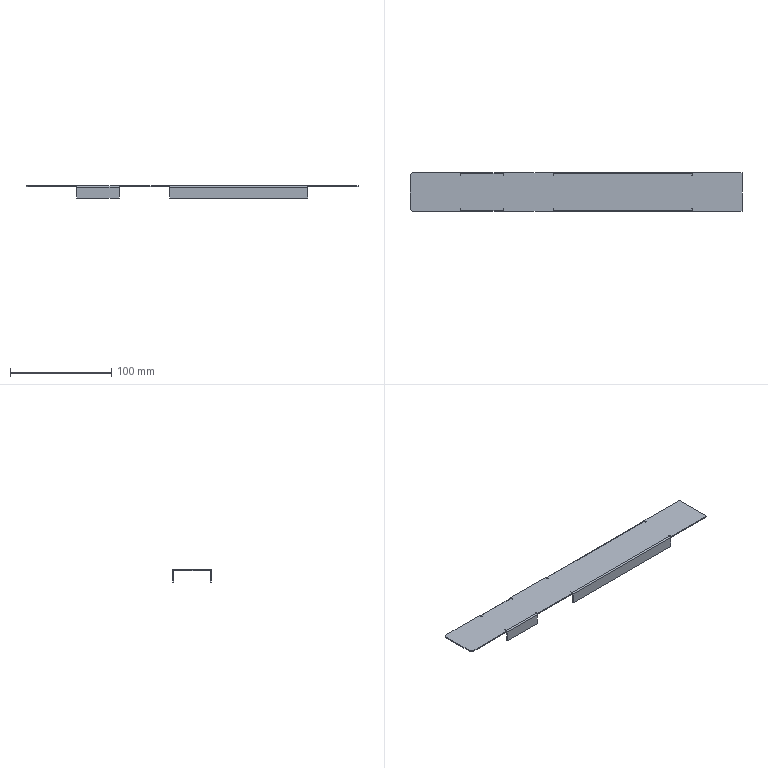Part | 1 solid | 72 faces | box 328 x 38 x 12 mm | volume 16268 mm3 | plane 64 | cylinder 8 | commonest cylinder face diameters 0.4 x4 2.4 x4